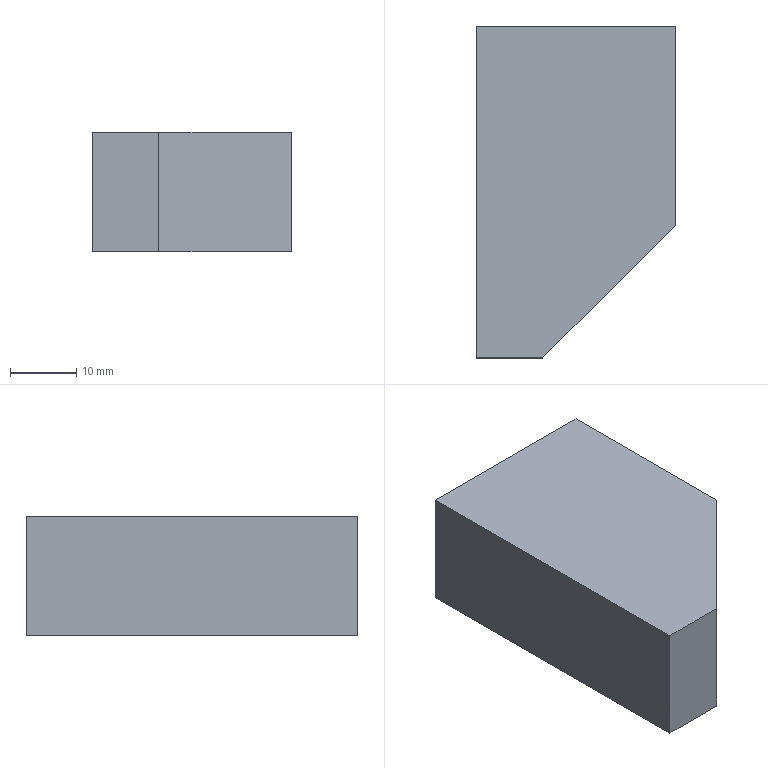Part | STEP file | Superstructure_3 | 1 solid | 7 faces | box 30 x 50 x 18 mm | volume 23400 mm3 | plane 7
STEP:
#1=CARTESIAN_POINT('',(0.,0.,0.));
#2=DIRECTION('',(0.,0.,1.));
#3=DIRECTION('',(1.,0.,0.));
#4=AXIS2_PLACEMENT_3D('',#1,#2,#3);
#5=CARTESIAN_POINT('',(15.,25.,-9.));
#6=VERTEX_POINT('',#5);
#7=CARTESIAN_POINT('',(15.,-5.,-9.));
#8=VERTEX_POINT('',#7);
#9=CARTESIAN_POINT('',(15.,25.,-9.));
#10=DIRECTION('',(0.,-1.,0.));
#11=VECTOR('',#10,1.);
#12=LINE('',#9,#11);
#13=CARTESIAN_POINT('',(-15.,25.,-9.));
#14=DIRECTION('',(0.,0.,1.));
#15=DIRECTION('',(1.,0.,0.));
#16=AXIS2_PLACEMENT_3D('',#13,#14,#15);
#17=PLANE('',#16);
#18=CARTESIAN_POINT('',(30.,0.));
#19=DIRECTION('',(0.,-1.));
#20=VECTOR('',#19,1.);
#21=LINE('',#18,#20);
#22=(GEOMETRIC_REPRESENTATION_CONTEXT(2)PARAMETRIC_REPRESENTATION_CONTEXT()REPRESENTATION_CONTEXT('',''));
#23=DEFINITIONAL_REPRESENTATION('',(#21),#22);
#24=PCURVE('',#17,#23);
#25=CARTESIAN_POINT('',(15.,25.,-9.));
#26=DIRECTION('',(-1.,0.,0.));
#27=DIRECTION('',(0.,0.,1.));
#28=AXIS2_PLACEMENT_3D('',#25,#26,#27);
#29=PLANE('',#28);
#30=CARTESIAN_POINT('',(0.,0.));
#31=DIRECTION('',(0.,-1.));
#32=VECTOR('',#31,1.);
#33=LINE('',#30,#32);
#34=(GEOMETRIC_REPRESENTATION_CONTEXT(2)PARAMETRIC_REPRESENTATION_CONTEXT()REPRESENTATION_CONTEXT('',''));
#35=DEFINITIONAL_REPRESENTATION('',(#33),#34);
#36=PCURVE('',#29,#35);
#37=SURFACE_CURVE('',#12,(#24,#36),.PCURVE_S1.);
#38=EDGE_CURVE('',#6,#8,#37,.T.);
#39=ORIENTED_EDGE('',*,*,#38,.F.);
#40=CARTESIAN_POINT('',(-15.,25.,-9.));
#41=VERTEX_POINT('',#40);
#42=CARTESIAN_POINT('',(-15.,25.,-9.));
#43=DIRECTION('',(1.,0.,0.));
#44=VECTOR('',#43,1.);
#45=LINE('',#42,#44);
#46=CARTESIAN_POINT('',(0.,0.));
#47=DIRECTION('',(1.,0.));
#48=VECTOR('',#47,1.);
#49=LINE('',#46,#48);
#50=(GEOMETRIC_REPRESENTATION_CONTEXT(2)PARAMETRIC_REPRESENTATION_CONTEXT()REPRESENTATION_CONTEXT('',''));
#51=DEFINITIONAL_REPRESENTATION('',(#49),#50);
#52=PCURVE('',#17,#51);
#53=CARTESIAN_POINT('',(0.,25.,0.));
#54=DIRECTION('',(0.,1.,0.));
#55=DIRECTION('',(0.,0.,1.));
#56=AXIS2_PLACEMENT_3D('',#53,#54,#55);
#57=PLANE('',#56);
#58=CARTESIAN_POINT('',(-9.,-15.));
#59=DIRECTION('',(0.,1.));
#60=VECTOR('',#59,1.);
#61=LINE('',#58,#60);
#62=(GEOMETRIC_REPRESENTATION_CONTEXT(2)PARAMETRIC_REPRESENTATION_CONTEXT()REPRESENTATION_CONTEXT('',''));
#63=DEFINITIONAL_REPRESENTATION('',(#61),#62);
#64=PCURVE('',#57,#63);
#65=SURFACE_CURVE('',#45,(#52,#64),.PCURVE_S1.);
#66=EDGE_CURVE('',#41,#6,#65,.T.);
#67=ORIENTED_EDGE('',*,*,#66,.F.);
#68=CARTESIAN_POINT('',(-15.,-25.,-9.));
#69=VERTEX_POINT('',#68);
#70=CARTESIAN_POINT('',(-15.,25.,-9.));
#71=DIRECTION('',(0.,-1.,0.));
#72=VECTOR('',#71,1.);
#73=LINE('',#70,#72);
#74=CARTESIAN_POINT('',(0.,0.));
#75=DIRECTION('',(0.,-1.));
#76=VECTOR('',#75,1.);
#77=LINE('',#74,#76);
#78=(GEOMETRIC_REPRESENTATION_CONTEXT(2)PARAMETRIC_REPRESENTATION_CONTEXT()REPRESENTATION_CONTEXT('',''));
#79=DEFINITIONAL_REPRESENTATION('',(#77),#78);
#80=PCURVE('',#17,#79);
#81=CARTESIAN_POINT('',(-15.,25.,9.));
#82=DIRECTION('',(1.,0.,0.));
#83=DIRECTION('',(0.,0.,-1.));
#84=AXIS2_PLACEMENT_3D('',#81,#82,#83);
#85=PLANE('',#84);
#86=CARTESIAN_POINT('',(18.,0.));
#87=DIRECTION('',(0.,-1.));
#88=VECTOR('',#87,1.);
#89=LINE('',#86,#88);
#90=(GEOMETRIC_REPRESENTATION_CONTEXT(2)PARAMETRIC_REPRESENTATION_CONTEXT()REPRESENTATION_CONTEXT('',''));
#91=DEFINITIONAL_REPRESENTATION('',(#89),#90);
#92=PCURVE('',#85,#91);
#93=SURFACE_CURVE('',#73,(#80,#92),.PCURVE_S1.);
#94=EDGE_CURVE('',#41,#69,#93,.T.);
#95=ORIENTED_EDGE('',*,*,#94,.T.);
#96=CARTESIAN_POINT('',(-5.,-25.,-9.));
#97=VERTEX_POINT('',#96);
#98=CARTESIAN_POINT('',(-15.,-25.,-9.));
#99=DIRECTION('',(1.,0.,0.));
#100=VECTOR('',#99,1.);
#101=LINE('',#98,#100);
#102=CARTESIAN_POINT('',(0.,-50.));
#103=DIRECTION('',(1.,0.));
#104=VECTOR('',#103,1.);
#105=LINE('',#102,#104);
#106=(GEOMETRIC_REPRESENTATION_CONTEXT(2)PARAMETRIC_REPRESENTATION_CONTEXT()REPRESENTATION_CONTEXT('',''));
#107=DEFINITIONAL_REPRESENTATION('',(#105),#106);
#108=PCURVE('',#17,#107);
#109=CARTESIAN_POINT('',(0.,-25.,0.));
#110=DIRECTION('',(0.,1.,0.));
#111=DIRECTION('',(0.,0.,1.));
#112=AXIS2_PLACEMENT_3D('',#109,#110,#111);
#113=PLANE('',#112);
#114=CARTESIAN_POINT('',(-9.,-15.));
#115=DIRECTION('',(0.,1.));
#116=VECTOR('',#115,1.);
#117=LINE('',#114,#116);
#118=(GEOMETRIC_REPRESENTATION_CONTEXT(2)PARAMETRIC_REPRESENTATION_CONTEXT()REPRESENTATION_CONTEXT('',''));
#119=DEFINITIONAL_REPRESENTATION('',(#117),#118);
#120=PCURVE('',#113,#119);
#121=SURFACE_CURVE('',#101,(#108,#120),.PCURVE_S1.);
#122=EDGE_CURVE('',#69,#97,#121,.T.);
#123=ORIENTED_EDGE('',*,*,#122,.T.);
#124=CARTESIAN_POINT('',(10.,-10.,-9.));
#125=DIRECTION('',(-0.7071,-0.7071,0.));
#126=VECTOR('',#125,1.);
#127=LINE('',#124,#126);
#128=CARTESIAN_POINT('',(25.,-35.));
#129=DIRECTION('',(-0.7071,-0.7071));
#130=VECTOR('',#129,1.);
#131=LINE('',#128,#130);
#132=(GEOMETRIC_REPRESENTATION_CONTEXT(2)PARAMETRIC_REPRESENTATION_CONTEXT()REPRESENTATION_CONTEXT('',''));
#133=DEFINITIONAL_REPRESENTATION('',(#131),#132);
#134=PCURVE('',#17,#133);
#135=CARTESIAN_POINT('',(5.,-15.,-9.));
#136=DIRECTION('',(0.7071,-0.7071,0.));
#137=DIRECTION('',(0.,0.,1.));
#138=AXIS2_PLACEMENT_3D('',#135,#136,#137);
#139=PLANE('',#138);
#140=CARTESIAN_POINT('',(0.,-7.071));
#141=DIRECTION('',(0.,1.));
#142=VECTOR('',#141,1.);
#143=LINE('',#140,#142);
#144=(GEOMETRIC_REPRESENTATION_CONTEXT(2)PARAMETRIC_REPRESENTATION_CONTEXT()REPRESENTATION_CONTEXT('',''));
#145=DEFINITIONAL_REPRESENTATION('',(#143),#144);
#146=PCURVE('',#139,#145);
#147=SURFACE_CURVE('',#127,(#134,#146),.PCURVE_S1.);
#148=EDGE_CURVE('',#8,#97,#147,.T.);
#149=ORIENTED_EDGE('',*,*,#148,.F.);
#150=EDGE_LOOP('',(#39,#67,#95,#123,#149));
#151=FACE_BOUND('',#150,.F.);
#152=ADVANCED_FACE('',(#151),#17,.F.);
#153=ORIENTED_EDGE('',*,*,#38,.T.);
#154=CARTESIAN_POINT('',(15.,-5.,9.));
#155=VERTEX_POINT('',#154);
#156=CARTESIAN_POINT('',(15.,-5.,-9.));
#157=DIRECTION('',(0.,0.,1.));
#158=VECTOR('',#157,1.);
#159=LINE('',#156,#158);
#160=CARTESIAN_POINT('',(0.,-30.));
#161=DIRECTION('',(1.,0.));
#162=VECTOR('',#161,1.);
#163=LINE('',#160,#162);
#164=(GEOMETRIC_REPRESENTATION_CONTEXT(2)PARAMETRIC_REPRESENTATION_CONTEXT()REPRESENTATION_CONTEXT('',''));
#165=DEFINITIONAL_REPRESENTATION('',(#163),#164);
#166=PCURVE('',#29,#165);
#167=CARTESIAN_POINT('',(0.,-14.142));
#168=DIRECTION('',(1.,0.));
#169=VECTOR('',#168,1.);
#170=LINE('',#167,#169);
#171=(GEOMETRIC_REPRESENTATION_CONTEXT(2)PARAMETRIC_REPRESENTATION_CONTEXT()REPRESENTATION_CONTEXT('',''));
#172=DEFINITIONAL_REPRESENTATION('',(#170),#171);
#173=PCURVE('',#139,#172);
#174=SURFACE_CURVE('',#159,(#166,#173),.PCURVE_S1.);
#175=EDGE_CURVE('',#8,#155,#174,.T.);
#176=ORIENTED_EDGE('',*,*,#175,.T.);
#177=CARTESIAN_POINT('',(15.,25.,9.));
#178=VERTEX_POINT('',#177);
#179=CARTESIAN_POINT('',(15.,25.,9.));
#180=DIRECTION('',(0.,-1.,0.));
#181=VECTOR('',#180,1.);
#182=LINE('',#179,#181);
#183=CARTESIAN_POINT('',(18.,0.));
#184=DIRECTION('',(0.,-1.));
#185=VECTOR('',#184,1.);
#186=LINE('',#183,#185);
#187=(GEOMETRIC_REPRESENTATION_CONTEXT(2)PARAMETRIC_REPRESENTATION_CONTEXT()REPRESENTATION_CONTEXT('',''));
#188=DEFINITIONAL_REPRESENTATION('',(#186),#187);
#189=PCURVE('',#29,#188);
#190=CARTESIAN_POINT('',(15.,25.,9.));
#191=DIRECTION('',(0.,0.,-1.));
#192=DIRECTION('',(-1.,0.,0.));
#193=AXIS2_PLACEMENT_3D('',#190,#191,#192);
#194=PLANE('',#193);
#195=CARTESIAN_POINT('',(0.,0.));
#196=DIRECTION('',(0.,-1.));
#197=VECTOR('',#196,1.);
#198=LINE('',#195,#197);
#199=(GEOMETRIC_REPRESENTATION_CONTEXT(2)PARAMETRIC_REPRESENTATION_CONTEXT()REPRESENTATION_CONTEXT('',''));
#200=DEFINITIONAL_REPRESENTATION('',(#198),#199);
#201=PCURVE('',#194,#200);
#202=SURFACE_CURVE('',#182,(#189,#201),.PCURVE_S1.);
#203=EDGE_CURVE('',#178,#155,#202,.T.);
#204=ORIENTED_EDGE('',*,*,#203,.F.);
#205=CARTESIAN_POINT('',(15.,25.,-9.));
#206=DIRECTION('',(0.,0.,1.));
#207=VECTOR('',#206,1.);
#208=LINE('',#205,#207);
#209=CARTESIAN_POINT('',(0.,0.));
#210=DIRECTION('',(1.,0.));
#211=VECTOR('',#210,1.);
#212=LINE('',#209,#211);
#213=(GEOMETRIC_REPRESENTATION_CONTEXT(2)PARAMETRIC_REPRESENTATION_CONTEXT()REPRESENTATION_CONTEXT('',''));
#214=DEFINITIONAL_REPRESENTATION('',(#212),#213);
#215=PCURVE('',#29,#214);
#216=CARTESIAN_POINT('',(-9.,15.));
#217=DIRECTION('',(1.,0.));
#218=VECTOR('',#217,1.);
#219=LINE('',#216,#218);
#220=(GEOMETRIC_REPRESENTATION_CONTEXT(2)PARAMETRIC_REPRESENTATION_CONTEXT()REPRESENTATION_CONTEXT('',''));
#221=DEFINITIONAL_REPRESENTATION('',(#219),#220);
#222=PCURVE('',#57,#221);
#223=SURFACE_CURVE('',#208,(#215,#222),.PCURVE_S1.);
#224=EDGE_CURVE('',#6,#178,#223,.T.);
#225=ORIENTED_EDGE('',*,*,#224,.F.);
#226=EDGE_LOOP('',(#153,#176,#204,#225));
#227=FACE_BOUND('',#226,.F.);
#228=ADVANCED_FACE('',(#227),#29,.F.);
#229=ORIENTED_EDGE('',*,*,#148,.F.);
#230=ORIENTED_EDGE('',*,*,#175,.T.);
#231=CARTESIAN_POINT('',(-5.,-25.,9.));
#232=VERTEX_POINT('',#231);
#233=CARTESIAN_POINT('',(17.5,-2.5,9.));
#234=DIRECTION('',(-0.7071,-0.7071,0.));
#235=VECTOR('',#234,1.);
#236=LINE('',#233,#235);
#237=CARTESIAN_POINT('',(18.,-17.678));
#238=DIRECTION('',(0.,1.));
#239=VECTOR('',#238,1.);
#240=LINE('',#237,#239);
#241=(GEOMETRIC_REPRESENTATION_CONTEXT(2)PARAMETRIC_REPRESENTATION_CONTEXT()REPRESENTATION_CONTEXT('',''));
#242=DEFINITIONAL_REPRESENTATION('',(#240),#241);
#243=PCURVE('',#139,#242);
#244=CARTESIAN_POINT('',(-2.5,-27.5));
#245=DIRECTION('',(0.7071,-0.7071));
#246=VECTOR('',#245,1.);
#247=LINE('',#244,#246);
#248=(GEOMETRIC_REPRESENTATION_CONTEXT(2)PARAMETRIC_REPRESENTATION_CONTEXT()REPRESENTATION_CONTEXT('',''));
#249=DEFINITIONAL_REPRESENTATION('',(#247),#248);
#250=PCURVE('',#194,#249);
#251=SURFACE_CURVE('',#236,(#243,#250),.PCURVE_S1.);
#252=EDGE_CURVE('',#155,#232,#251,.T.);
#253=ORIENTED_EDGE('',*,*,#252,.T.);
#254=CARTESIAN_POINT('',(-5.,-25.,-9.));
#255=DIRECTION('',(0.,0.,1.));
#256=VECTOR('',#255,1.);
#257=LINE('',#254,#256);
#258=CARTESIAN_POINT('',(0.,14.142));
#259=DIRECTION('',(1.,0.));
#260=VECTOR('',#259,1.);
#261=LINE('',#258,#260);
#262=(GEOMETRIC_REPRESENTATION_CONTEXT(2)PARAMETRIC_REPRESENTATION_CONTEXT()REPRESENTATION_CONTEXT('',''));
#263=DEFINITIONAL_REPRESENTATION('',(#261),#262);
#264=PCURVE('',#139,#263);
#265=CARTESIAN_POINT('',(-9.,-5.));
#266=DIRECTION('',(1.,0.));
#267=VECTOR('',#266,1.);
#268=LINE('',#265,#267);
#269=(GEOMETRIC_REPRESENTATION_CONTEXT(2)PARAMETRIC_REPRESENTATION_CONTEXT()REPRESENTATION_CONTEXT('',''));
#270=DEFINITIONAL_REPRESENTATION('',(#268),#269);
#271=PCURVE('',#113,#270);
#272=SURFACE_CURVE('',#257,(#264,#271),.PCURVE_S1.);
#273=EDGE_CURVE('',#97,#232,#272,.T.);
#274=ORIENTED_EDGE('',*,*,#273,.F.);
#275=EDGE_LOOP('',(#229,#230,#253,#274));
#276=FACE_BOUND('',#275,.T.);
#277=ADVANCED_FACE('',(#276),#139,.T.);
#278=CARTESIAN_POINT('',(-15.,25.,9.));
#279=VERTEX_POINT('',#278);
#280=CARTESIAN_POINT('',(-15.,25.,9.));
#281=DIRECTION('',(0.,0.,-1.));
#282=VECTOR('',#281,1.);
#283=LINE('',#280,#282);
#284=CARTESIAN_POINT('',(9.,-15.));
#285=DIRECTION('',(-1.,0.));
#286=VECTOR('',#285,1.);
#287=LINE('',#284,#286);
#288=(GEOMETRIC_REPRESENTATION_CONTEXT(2)PARAMETRIC_REPRESENTATION_CONTEXT()REPRESENTATION_CONTEXT('',''));
#289=DEFINITIONAL_REPRESENTATION('',(#287),#288);
#290=PCURVE('',#57,#289);
#291=CARTESIAN_POINT('',(0.,0.));
#292=DIRECTION('',(1.,0.));
#293=VECTOR('',#292,1.);
#294=LINE('',#291,#293);
#295=(GEOMETRIC_REPRESENTATION_CONTEXT(2)PARAMETRIC_REPRESENTATION_CONTEXT()REPRESENTATION_CONTEXT('',''));
#296=DEFINITIONAL_REPRESENTATION('',(#294),#295);
#297=PCURVE('',#85,#296);
#298=SURFACE_CURVE('',#283,(#290,#297),.PCURVE_S1.);
#299=EDGE_CURVE('',#279,#41,#298,.T.);
#300=ORIENTED_EDGE('',*,*,#299,.T.);
#301=ORIENTED_EDGE('',*,*,#66,.T.);
#302=ORIENTED_EDGE('',*,*,#224,.T.);
#303=CARTESIAN_POINT('',(15.,25.,9.));
#304=DIRECTION('',(-1.,0.,0.));
#305=VECTOR('',#304,1.);
#306=LINE('',#303,#305);
#307=CARTESIAN_POINT('',(9.,15.));
#308=DIRECTION('',(0.,-1.));
#309=VECTOR('',#308,1.);
#310=LINE('',#307,#309);
#311=(GEOMETRIC_REPRESENTATION_CONTEXT(2)PARAMETRIC_REPRESENTATION_CONTEXT()REPRESENTATION_CONTEXT('',''));
#312=DEFINITIONAL_REPRESENTATION('',(#310),#311);
#313=PCURVE('',#57,#312);
#314=CARTESIAN_POINT('',(0.,0.));
#315=DIRECTION('',(1.,0.));
#316=VECTOR('',#315,1.);
#317=LINE('',#314,#316);
#318=(GEOMETRIC_REPRESENTATION_CONTEXT(2)PARAMETRIC_REPRESENTATION_CONTEXT()REPRESENTATION_CONTEXT('',''));
#319=DEFINITIONAL_REPRESENTATION('',(#317),#318);
#320=PCURVE('',#194,#319);
#321=SURFACE_CURVE('',#306,(#313,#320),.PCURVE_S1.);
#322=EDGE_CURVE('',#178,#279,#321,.T.);
#323=ORIENTED_EDGE('',*,*,#322,.T.);
#324=EDGE_LOOP('',(#300,#301,#302,#323));
#325=FACE_BOUND('',#324,.F.);
#326=ADVANCED_FACE('',(#325),#57,.T.);
#327=ORIENTED_EDGE('',*,*,#122,.F.);
#328=CARTESIAN_POINT('',(-15.,-25.,9.));
#329=VERTEX_POINT('',#328);
#330=CARTESIAN_POINT('',(-15.,-25.,9.));
#331=DIRECTION('',(0.,0.,-1.));
#332=VECTOR('',#331,1.);
#333=LINE('',#330,#332);
#334=CARTESIAN_POINT('',(9.,-15.));
#335=DIRECTION('',(-1.,0.));
#336=VECTOR('',#335,1.);
#337=LINE('',#334,#336);
#338=(GEOMETRIC_REPRESENTATION_CONTEXT(2)PARAMETRIC_REPRESENTATION_CONTEXT()REPRESENTATION_CONTEXT('',''));
#339=DEFINITIONAL_REPRESENTATION('',(#337),#338);
#340=PCURVE('',#113,#339);
#341=CARTESIAN_POINT('',(0.,-50.));
#342=DIRECTION('',(1.,0.));
#343=VECTOR('',#342,1.);
#344=LINE('',#341,#343);
#345=(GEOMETRIC_REPRESENTATION_CONTEXT(2)PARAMETRIC_REPRESENTATION_CONTEXT()REPRESENTATION_CONTEXT('',''));
#346=DEFINITIONAL_REPRESENTATION('',(#344),#345);
#347=PCURVE('',#85,#346);
#348=SURFACE_CURVE('',#333,(#340,#347),.PCURVE_S1.);
#349=EDGE_CURVE('',#329,#69,#348,.T.);
#350=ORIENTED_EDGE('',*,*,#349,.F.);
#351=CARTESIAN_POINT('',(15.,-25.,9.));
#352=DIRECTION('',(-1.,0.,0.));
#353=VECTOR('',#352,1.);
#354=LINE('',#351,#353);
#355=CARTESIAN_POINT('',(9.,15.));
#356=DIRECTION('',(0.,-1.));
#357=VECTOR('',#356,1.);
#358=LINE('',#355,#357);
#359=(GEOMETRIC_REPRESENTATION_CONTEXT(2)PARAMETRIC_REPRESENTATION_CONTEXT()REPRESENTATION_CONTEXT('',''));
#360=DEFINITIONAL_REPRESENTATION('',(#358),#359);
#361=PCURVE('',#113,#360);
#362=CARTESIAN_POINT('',(0.,-50.));
#363=DIRECTION('',(1.,0.));
#364=VECTOR('',#363,1.);
#365=LINE('',#362,#364);
#366=(GEOMETRIC_REPRESENTATION_CONTEXT(2)PARAMETRIC_REPRESENTATION_CONTEXT()REPRESENTATION_CONTEXT('',''));
#367=DEFINITIONAL_REPRESENTATION('',(#365),#366);
#368=PCURVE('',#194,#367);
#369=SURFACE_CURVE('',#354,(#361,#368),.PCURVE_S1.);
#370=EDGE_CURVE('',#232,#329,#369,.T.);
#371=ORIENTED_EDGE('',*,*,#370,.F.);
#372=ORIENTED_EDGE('',*,*,#273,.F.);
#373=EDGE_LOOP('',(#327,#350,#371,#372));
#374=FACE_BOUND('',#373,.F.);
#375=ADVANCED_FACE('',(#374),#113,.F.);
#376=CARTESIAN_POINT('',(-15.,25.,9.));
#377=DIRECTION('',(0.,-1.,0.));
#378=VECTOR('',#377,1.);
#379=LINE('',#376,#378);
#380=CARTESIAN_POINT('',(0.,0.));
#381=DIRECTION('',(0.,-1.));
#382=VECTOR('',#381,1.);
#383=LINE('',#380,#382);
#384=(GEOMETRIC_REPRESENTATION_CONTEXT(2)PARAMETRIC_REPRESENTATION_CONTEXT()REPRESENTATION_CONTEXT('',''));
#385=DEFINITIONAL_REPRESENTATION('',(#383),#384);
#386=PCURVE('',#85,#385);
#387=CARTESIAN_POINT('',(30.,0.));
#388=DIRECTION('',(0.,-1.));
#389=VECTOR('',#388,1.);
#390=LINE('',#387,#389);
#391=(GEOMETRIC_REPRESENTATION_CONTEXT(2)PARAMETRIC_REPRESENTATION_CONTEXT()REPRESENTATION_CONTEXT('',''));
#392=DEFINITIONAL_REPRESENTATION('',(#390),#391);
#393=PCURVE('',#194,#392);
#394=SURFACE_CURVE('',#379,(#386,#393),.PCURVE_S1.);
#395=EDGE_CURVE('',#279,#329,#394,.T.);
#396=ORIENTED_EDGE('',*,*,#395,.T.);
#397=ORIENTED_EDGE('',*,*,#349,.T.);
#398=ORIENTED_EDGE('',*,*,#94,.F.);
#399=ORIENTED_EDGE('',*,*,#299,.F.);
#400=EDGE_LOOP('',(#396,#397,#398,#399));
#401=FACE_BOUND('',#400,.F.);
#402=ADVANCED_FACE('',(#401),#85,.F.);
#403=ORIENTED_EDGE('',*,*,#203,.T.);
#404=ORIENTED_EDGE('',*,*,#252,.T.);
#405=ORIENTED_EDGE('',*,*,#370,.T.);
#406=ORIENTED_EDGE('',*,*,#395,.F.);
#407=ORIENTED_EDGE('',*,*,#322,.F.);
#408=EDGE_LOOP('',(#403,#404,#405,#406,#407));
#409=FACE_BOUND('',#408,.F.);
#410=ADVANCED_FACE('',(#409),#194,.F.);
#411=CLOSED_SHELL('',(#152,#228,#277,#326,#375,#402,#410));
#412=MANIFOLD_SOLID_BREP('',#411);
#413=(LENGTH_UNIT()NAMED_UNIT(*)SI_UNIT(.MILLI.,.METRE.));
#414=UNCERTAINTY_MEASURE_WITH_UNIT(LENGTH_MEASURE(0.0000001),#413,'','');
#415=(NAMED_UNIT(*)PLANE_ANGLE_UNIT()SI_UNIT($,.RADIAN.));
#416=(NAMED_UNIT(*)SI_UNIT($,.STERADIAN.)SOLID_ANGLE_UNIT());
#417=(GEOMETRIC_REPRESENTATION_CONTEXT(3)GLOBAL_UNCERTAINTY_ASSIGNED_CONTEXT((#414))GLOBAL_UNIT_ASSIGNED_CONTEXT((#413,#415,#416))REPRESENTATION_CONTEXT('',''));
#418=ADVANCED_BREP_SHAPE_REPRESENTATION('',(#4,#412),#417);